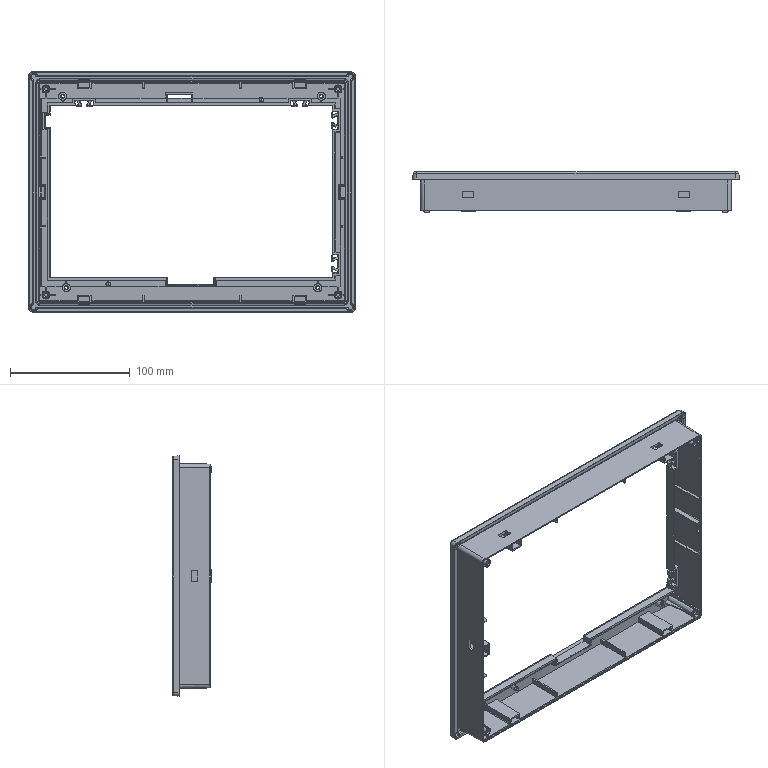Part | SolidWorks | features BaseBody 1 | 1 solid | 777 faces | box 272.622 x 33.34 x 200.622 mm | volume 144122 mm3 | plane 511 | cylinder 178 | cone 52 | spline 36 | commonest cylinder face diameters 1 x66 2 x58 2.5 x16 0.4 x8 3 x8 6 x8